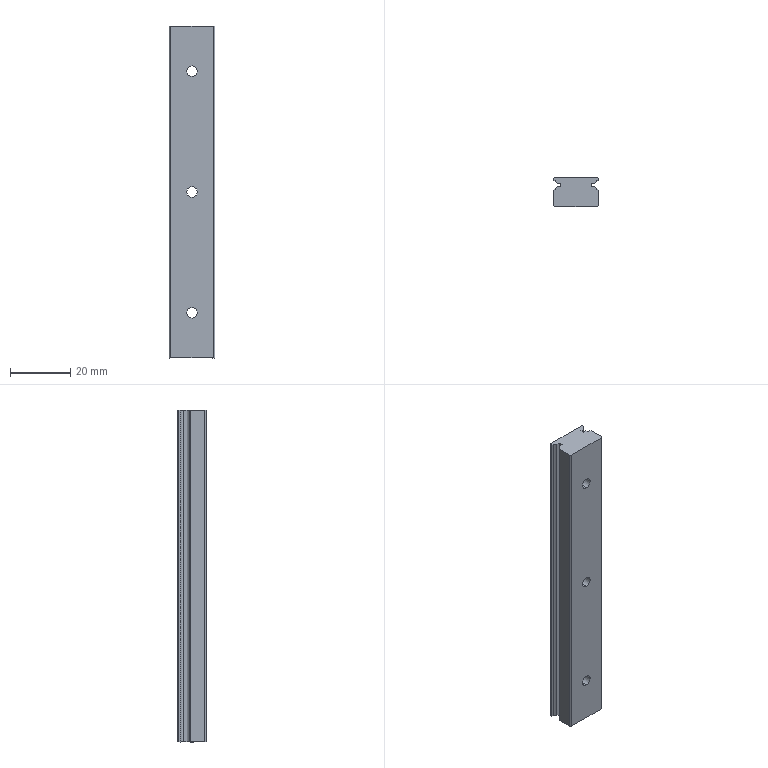Part | SolidWorks | features BaseBody 1 | 1 solid | 41 faces | box 15 x 9.5 x 110 mm | volume 14060 mm3 | plane 25 | cylinder 16 | commonest cylinder face diameters 3.5 x10 6 x6
STEP:
#1=CARTESIAN_POINT('',(0.,5.,-38.25));
#2=VERTEX_POINT('',#1);
#3=CARTESIAN_POINT('',(0.,5.,-41.75));
#4=VERTEX_POINT('',#3);
#5=CARTESIAN_POINT('',(0.,5.,-40.));
#6=DIRECTION('',(0.,-1.,0.));
#7=DIRECTION('',(0.,0.,-1.));
#8=AXIS2_PLACEMENT_3D('',#5,#6,#7);
#9=CIRCLE('',#8,1.75);
#10=EDGE_CURVE('',#2,#4,#9,.T.);
#11=ORIENTED_EDGE('',*,*,#10,.F.);
#12=CARTESIAN_POINT('',(0.,0.,-38.25));
#13=VERTEX_POINT('',#12);
#14=CARTESIAN_POINT('',(0.,2.5,-38.25));
#15=DIRECTION('',(0.,-1.,0.));
#16=VECTOR('',#15,1000.);
#17=LINE('',#14,#16);
#18=EDGE_CURVE('',#2,#13,#17,.T.);
#19=ORIENTED_EDGE('',*,*,#18,.T.);
#20=CARTESIAN_POINT('',(0.,0.,-41.75));
#21=VERTEX_POINT('',#20);
#22=CARTESIAN_POINT('',(0.,0.,-40.));
#23=DIRECTION('',(0.,1.,0.));
#24=DIRECTION('',(0.,0.,-1.));
#25=AXIS2_PLACEMENT_3D('',#22,#23,#24);
#26=CIRCLE('',#25,1.75);
#27=EDGE_CURVE('',#21,#13,#26,.T.);
#28=ORIENTED_EDGE('',*,*,#27,.F.);
#29=CARTESIAN_POINT('',(0.,2.5,-41.75));
#30=DIRECTION('',(0.,-1.,0.));
#31=VECTOR('',#30,1000.);
#32=LINE('',#29,#31);
#33=EDGE_CURVE('',#4,#21,#32,.T.);
#34=ORIENTED_EDGE('',*,*,#33,.F.);
#35=EDGE_LOOP('',(#11,#19,#28,#34));
#36=FACE_OUTER_BOUND('',#35,.T.);
#37=CARTESIAN_POINT('',(0.,2.5,-40.));
#38=DIRECTION('',(0.,-1.,0.));
#39=DIRECTION('',(0.,0.,-1.));
#40=AXIS2_PLACEMENT_3D('',#37,#38,#39);
#41=CYLINDRICAL_SURFACE('',#40,1.75);
#42=ADVANCED_FACE('',(#36),#41,.F.);
#43=CARTESIAN_POINT('',(0.,5.,41.75));
#44=VERTEX_POINT('',#43);
#45=CARTESIAN_POINT('',(0.,5.,38.25));
#46=VERTEX_POINT('',#45);
#47=CARTESIAN_POINT('',(0.,5.,40.));
#48=DIRECTION('',(0.,-1.,0.));
#49=DIRECTION('',(0.,0.,-1.));
#50=AXIS2_PLACEMENT_3D('',#47,#48,#49);
#51=CIRCLE('',#50,1.75);
#52=EDGE_CURVE('',#44,#46,#51,.T.);
#53=ORIENTED_EDGE('',*,*,#52,.F.);
#54=CARTESIAN_POINT('',(0.,0.,41.75));
#55=VERTEX_POINT('',#54);
#56=CARTESIAN_POINT('',(0.,2.5,41.75));
#57=DIRECTION('',(0.,-1.,0.));
#58=VECTOR('',#57,1000.);
#59=LINE('',#56,#58);
#60=EDGE_CURVE('',#44,#55,#59,.T.);
#61=ORIENTED_EDGE('',*,*,#60,.T.);
#62=CARTESIAN_POINT('',(0.,0.,38.25));
#63=VERTEX_POINT('',#62);
#64=CARTESIAN_POINT('',(0.,0.,40.));
#65=DIRECTION('',(0.,1.,0.));
#66=DIRECTION('',(0.,0.,-1.));
#67=AXIS2_PLACEMENT_3D('',#64,#65,#66);
#68=CIRCLE('',#67,1.75);
#69=EDGE_CURVE('',#63,#55,#68,.T.);
#70=ORIENTED_EDGE('',*,*,#69,.F.);
#71=CARTESIAN_POINT('',(0.,2.5,38.25));
#72=DIRECTION('',(0.,-1.,0.));
#73=VECTOR('',#72,1000.);
#74=LINE('',#71,#73);
#75=EDGE_CURVE('',#46,#63,#74,.T.);
#76=ORIENTED_EDGE('',*,*,#75,.F.);
#77=EDGE_LOOP('',(#53,#61,#70,#76));
#78=FACE_OUTER_BOUND('',#77,.T.);
#79=CARTESIAN_POINT('',(0.,2.5,40.));
#80=DIRECTION('',(0.,-1.,0.));
#81=DIRECTION('',(0.,0.,-1.));
#82=AXIS2_PLACEMENT_3D('',#79,#80,#81);
#83=CYLINDRICAL_SURFACE('',#82,1.75);
#84=ADVANCED_FACE('',(#78),#83,.F.);
#85=CARTESIAN_POINT('',(0.,5.,1.75));
#86=VERTEX_POINT('',#85);
#87=CARTESIAN_POINT('',(0.,5.,-1.75));
#88=VERTEX_POINT('',#87);
#89=CARTESIAN_POINT('',(0.,5.,0.));
#90=DIRECTION('',(0.,-1.,0.));
#91=DIRECTION('',(0.,0.,-1.));
#92=AXIS2_PLACEMENT_3D('',#89,#90,#91);
#93=CIRCLE('',#92,1.75);
#94=EDGE_CURVE('',#86,#88,#93,.T.);
#95=ORIENTED_EDGE('',*,*,#94,.F.);
#96=CARTESIAN_POINT('',(0.,0.,1.75));
#97=VERTEX_POINT('',#96);
#98=CARTESIAN_POINT('',(0.,2.5,1.75));
#99=DIRECTION('',(0.,-1.,0.));
#100=VECTOR('',#99,1000.);
#101=LINE('',#98,#100);
#102=EDGE_CURVE('',#86,#97,#101,.T.);
#103=ORIENTED_EDGE('',*,*,#102,.T.);
#104=CARTESIAN_POINT('',(0.,0.,-1.75));
#105=VERTEX_POINT('',#104);
#106=CARTESIAN_POINT('',(0.,0.,0.));
#107=DIRECTION('',(0.,1.,0.));
#108=DIRECTION('',(0.,0.,-1.));
#109=AXIS2_PLACEMENT_3D('',#106,#107,#108);
#110=CIRCLE('',#109,1.75);
#111=EDGE_CURVE('',#105,#97,#110,.T.);
#112=ORIENTED_EDGE('',*,*,#111,.F.);
#113=CARTESIAN_POINT('',(0.,2.5,-1.75));
#114=DIRECTION('',(0.,-1.,0.));
#115=VECTOR('',#114,1000.);
#116=LINE('',#113,#115);
#117=EDGE_CURVE('',#88,#105,#116,.T.);
#118=ORIENTED_EDGE('',*,*,#117,.F.);
#119=EDGE_LOOP('',(#95,#103,#112,#118));
#120=FACE_OUTER_BOUND('',#119,.T.);
#121=CARTESIAN_POINT('',(0.,2.5,0.));
#122=DIRECTION('',(0.,-1.,0.));
#123=DIRECTION('',(0.,0.,-1.));
#124=AXIS2_PLACEMENT_3D('',#121,#122,#123);
#125=CYLINDRICAL_SURFACE('',#124,1.75);
#126=ADVANCED_FACE('',(#120),#125,.F.);
#127=CARTESIAN_POINT('',(0.,9.5,-37.));
#128=VERTEX_POINT('',#127);
#129=CARTESIAN_POINT('',(0.,9.5,-43.));
#130=VERTEX_POINT('',#129);
#131=CARTESIAN_POINT('',(0.,9.5,-40.));
#132=DIRECTION('',(0.,-1.,0.));
#133=DIRECTION('',(0.,0.,-1.));
#134=AXIS2_PLACEMENT_3D('',#131,#132,#133);
#135=CIRCLE('',#134,3.);
#136=EDGE_CURVE('',#128,#130,#135,.T.);
#137=ORIENTED_EDGE('',*,*,#136,.F.);
#138=CARTESIAN_POINT('',(0.,5.,-37.));
#139=VERTEX_POINT('',#138);
#140=CARTESIAN_POINT('',(0.,7.25,-37.));
#141=DIRECTION('',(0.,-1.,0.));
#142=VECTOR('',#141,1000.);
#143=LINE('',#140,#142);
#144=EDGE_CURVE('',#128,#139,#143,.T.);
#145=ORIENTED_EDGE('',*,*,#144,.T.);
#146=CARTESIAN_POINT('',(0.,5.,-43.));
#147=VERTEX_POINT('',#146);
#148=CARTESIAN_POINT('',(0.,5.,-40.));
#149=DIRECTION('',(0.,-1.,0.));
#150=DIRECTION('',(0.,0.,-1.));
#151=AXIS2_PLACEMENT_3D('',#148,#149,#150);
#152=CIRCLE('',#151,3.);
#153=EDGE_CURVE('',#139,#147,#152,.T.);
#154=ORIENTED_EDGE('',*,*,#153,.T.);
#155=CARTESIAN_POINT('',(0.,7.25,-43.));
#156=DIRECTION('',(0.,-1.,0.));
#157=VECTOR('',#156,1000.);
#158=LINE('',#155,#157);
#159=EDGE_CURVE('',#130,#147,#158,.T.);
#160=ORIENTED_EDGE('',*,*,#159,.F.);
#161=EDGE_LOOP('',(#137,#145,#154,#160));
#162=FACE_OUTER_BOUND('',#161,.T.);
#163=CARTESIAN_POINT('',(0.,7.25,-40.));
#164=DIRECTION('',(0.,-1.,0.));
#165=DIRECTION('',(0.,0.,-1.));
#166=AXIS2_PLACEMENT_3D('',#163,#164,#165);
#167=CYLINDRICAL_SURFACE('',#166,3.);
#168=ADVANCED_FACE('',(#162),#167,.F.);
#169=CARTESIAN_POINT('',(0.,9.5,43.));
#170=VERTEX_POINT('',#169);
#171=CARTESIAN_POINT('',(0.,9.5,37.));
#172=VERTEX_POINT('',#171);
#173=CARTESIAN_POINT('',(0.,9.5,40.));
#174=DIRECTION('',(0.,-1.,0.));
#175=DIRECTION('',(0.,0.,-1.));
#176=AXIS2_PLACEMENT_3D('',#173,#174,#175);
#177=CIRCLE('',#176,3.);
#178=EDGE_CURVE('',#170,#172,#177,.T.);
#179=ORIENTED_EDGE('',*,*,#178,.F.);
#180=CARTESIAN_POINT('',(0.,5.,43.));
#181=VERTEX_POINT('',#180);
#182=CARTESIAN_POINT('',(0.,7.25,43.));
#183=DIRECTION('',(0.,-1.,0.));
#184=VECTOR('',#183,1000.);
#185=LINE('',#182,#184);
#186=EDGE_CURVE('',#170,#181,#185,.T.);
#187=ORIENTED_EDGE('',*,*,#186,.T.);
#188=CARTESIAN_POINT('',(0.,5.,37.));
#189=VERTEX_POINT('',#188);
#190=CARTESIAN_POINT('',(0.,5.,40.));
#191=DIRECTION('',(0.,-1.,0.));
#192=DIRECTION('',(0.,0.,-1.));
#193=AXIS2_PLACEMENT_3D('',#190,#191,#192);
#194=CIRCLE('',#193,3.);
#195=EDGE_CURVE('',#181,#189,#194,.T.);
#196=ORIENTED_EDGE('',*,*,#195,.T.);
#197=CARTESIAN_POINT('',(0.,7.25,37.));
#198=DIRECTION('',(0.,-1.,0.));
#199=VECTOR('',#198,1000.);
#200=LINE('',#197,#199);
#201=EDGE_CURVE('',#172,#189,#200,.T.);
#202=ORIENTED_EDGE('',*,*,#201,.F.);
#203=EDGE_LOOP('',(#179,#187,#196,#202));
#204=FACE_OUTER_BOUND('',#203,.T.);
#205=CARTESIAN_POINT('',(0.,7.25,40.));
#206=DIRECTION('',(0.,-1.,0.));
#207=DIRECTION('',(0.,0.,-1.));
#208=AXIS2_PLACEMENT_3D('',#205,#206,#207);
#209=CYLINDRICAL_SURFACE('',#208,3.);
#210=ADVANCED_FACE('',(#204),#209,.F.);
#211=CARTESIAN_POINT('',(0.,9.5,3.));
#212=VERTEX_POINT('',#211);
#213=CARTESIAN_POINT('',(0.,9.5,-3.));
#214=VERTEX_POINT('',#213);
#215=CARTESIAN_POINT('',(0.,9.5,0.));
#216=DIRECTION('',(0.,-1.,0.));
#217=DIRECTION('',(0.,0.,-1.));
#218=AXIS2_PLACEMENT_3D('',#215,#216,#217);
#219=CIRCLE('',#218,3.);
#220=EDGE_CURVE('',#212,#214,#219,.T.);
#221=ORIENTED_EDGE('',*,*,#220,.F.);
#222=CARTESIAN_POINT('',(0.,5.,3.));
#223=VERTEX_POINT('',#222);
#224=CARTESIAN_POINT('',(0.,7.25,3.));
#225=DIRECTION('',(0.,-1.,0.));
#226=VECTOR('',#225,1000.);
#227=LINE('',#224,#226);
#228=EDGE_CURVE('',#212,#223,#227,.T.);
#229=ORIENTED_EDGE('',*,*,#228,.T.);
#230=CARTESIAN_POINT('',(0.,5.,-3.));
#231=VERTEX_POINT('',#230);
#232=CARTESIAN_POINT('',(0.,5.,0.));
#233=DIRECTION('',(0.,-1.,0.));
#234=DIRECTION('',(0.,0.,-1.));
#235=AXIS2_PLACEMENT_3D('',#232,#233,#234);
#236=CIRCLE('',#235,3.);
#237=EDGE_CURVE('',#223,#231,#236,.T.);
#238=ORIENTED_EDGE('',*,*,#237,.T.);
#239=CARTESIAN_POINT('',(0.,7.25,-3.));
#240=DIRECTION('',(0.,-1.,0.));
#241=VECTOR('',#240,1000.);
#242=LINE('',#239,#241);
#243=EDGE_CURVE('',#214,#231,#242,.T.);
#244=ORIENTED_EDGE('',*,*,#243,.F.);
#245=EDGE_LOOP('',(#221,#229,#238,#244));
#246=FACE_OUTER_BOUND('',#245,.T.);
#247=CARTESIAN_POINT('',(0.,7.25,0.));
#248=DIRECTION('',(0.,-1.,0.));
#249=DIRECTION('',(0.,0.,-1.));
#250=AXIS2_PLACEMENT_3D('',#247,#248,#249);
#251=CYLINDRICAL_SURFACE('',#250,3.);
#252=ADVANCED_FACE('',(#246),#251,.F.);
#253=CARTESIAN_POINT('',(7.,0.,55.));
#254=VERTEX_POINT('',#253);
#255=CARTESIAN_POINT('',(-7.,0.,55.));
#256=VERTEX_POINT('',#255);
#257=CARTESIAN_POINT('',(-7.,0.,55.));
#258=DIRECTION('',(-1.,0.,0.));
#259=VECTOR('',#258,1000.);
#260=LINE('',#257,#259);
#261=EDGE_CURVE('',#254,#256,#260,.T.);
#262=ORIENTED_EDGE('',*,*,#261,.T.);
#263=CARTESIAN_POINT('',(-7.,0.,-55.));
#264=VERTEX_POINT('',#263);
#265=CARTESIAN_POINT('',(-7.,0.,55.));
#266=DIRECTION('',(0.,0.,-1.));
#267=VECTOR('',#266,1000.);
#268=LINE('',#265,#267);
#269=EDGE_CURVE('',#256,#264,#268,.T.);
#270=ORIENTED_EDGE('',*,*,#269,.T.);
#271=CARTESIAN_POINT('',(7.,0.,-55.));
#272=VERTEX_POINT('',#271);
#273=CARTESIAN_POINT('',(-7.,0.,-55.));
#274=DIRECTION('',(1.,0.,0.));
#275=VECTOR('',#274,1000.);
#276=LINE('',#273,#275);
#277=EDGE_CURVE('',#264,#272,#276,.T.);
#278=ORIENTED_EDGE('',*,*,#277,.T.);
#279=CARTESIAN_POINT('',(7.,0.,55.));
#280=DIRECTION('',(0.,0.,1.));
#281=VECTOR('',#280,1000.);
#282=LINE('',#279,#281);
#283=EDGE_CURVE('',#272,#254,#282,.T.);
#284=ORIENTED_EDGE('',*,*,#283,.T.);
#285=EDGE_LOOP('',(#262,#270,#278,#284));
#286=FACE_OUTER_BOUND('',#285,.T.);
#287=ORIENTED_EDGE('',*,*,#27,.T.);
#288=CARTESIAN_POINT('',(0.,0.,-40.));
#289=DIRECTION('',(0.,1.,0.));
#290=DIRECTION('',(0.,0.,-1.));
#291=AXIS2_PLACEMENT_3D('',#288,#289,#290);
#292=CIRCLE('',#291,1.75);
#293=EDGE_CURVE('',#13,#21,#292,.T.);
#294=ORIENTED_EDGE('',*,*,#293,.T.);
#295=EDGE_LOOP('',(#287,#294));
#296=FACE_BOUND('',#295,.T.);
#297=ORIENTED_EDGE('',*,*,#69,.T.);
#298=CARTESIAN_POINT('',(0.,0.,40.));
#299=DIRECTION('',(0.,1.,0.));
#300=DIRECTION('',(0.,0.,-1.));
#301=AXIS2_PLACEMENT_3D('',#298,#299,#300);
#302=CIRCLE('',#301,1.75);
#303=EDGE_CURVE('',#55,#63,#302,.T.);
#304=ORIENTED_EDGE('',*,*,#303,.T.);
#305=EDGE_LOOP('',(#297,#304));
#306=FACE_BOUND('',#305,.T.);
#307=ORIENTED_EDGE('',*,*,#111,.T.);
#308=CARTESIAN_POINT('',(0.,0.,0.));
#309=DIRECTION('',(0.,1.,0.));
#310=DIRECTION('',(0.,0.,-1.));
#311=AXIS2_PLACEMENT_3D('',#308,#309,#310);
#312=CIRCLE('',#311,1.75);
#313=EDGE_CURVE('',#97,#105,#312,.T.);
#314=ORIENTED_EDGE('',*,*,#313,.T.);
#315=EDGE_LOOP('',(#307,#314));
#316=FACE_BOUND('',#315,.T.);
#317=CARTESIAN_POINT('',(-7.,0.,55.));
#318=DIRECTION('',(0.,-1.,0.));
#319=DIRECTION('',(0.,0.,-1.));
#320=AXIS2_PLACEMENT_3D('',#317,#318,#319);
#321=PLANE('',#320);
#322=ADVANCED_FACE('',(#286,#296,#306,#316),#321,.T.);
#323=CARTESIAN_POINT('',(-7.5,0.5,55.));
#324=VERTEX_POINT('',#323);
#325=CARTESIAN_POINT('',(-7.5,0.5,55.));
#326=DIRECTION('',(-0.7071,0.7071,0.));
#327=VECTOR('',#326,1000.);
#328=LINE('',#325,#327);
#329=EDGE_CURVE('',#256,#324,#328,.T.);
#330=ORIENTED_EDGE('',*,*,#329,.T.);
#331=CARTESIAN_POINT('',(-7.5,0.5,-55.));
#332=VERTEX_POINT('',#331);
#333=CARTESIAN_POINT('',(-7.5,0.5,55.));
#334=DIRECTION('',(0.,0.,-1.));
#335=VECTOR('',#334,1000.);
#336=LINE('',#333,#335);
#337=EDGE_CURVE('',#324,#332,#336,.T.);
#338=ORIENTED_EDGE('',*,*,#337,.T.);
#339=CARTESIAN_POINT('',(-7.5,0.5,-55.));
#340=DIRECTION('',(0.7071,-0.7071,0.));
#341=VECTOR('',#340,1000.);
#342=LINE('',#339,#341);
#343=EDGE_CURVE('',#332,#264,#342,.T.);
#344=ORIENTED_EDGE('',*,*,#343,.T.);
#345=ORIENTED_EDGE('',*,*,#269,.F.);
#346=EDGE_LOOP('',(#330,#338,#344,#345));
#347=FACE_OUTER_BOUND('',#346,.T.);
#348=CARTESIAN_POINT('',(-7.5,0.5,55.));
#349=DIRECTION('',(-0.7071,-0.7071,0.));
#350=DIRECTION('',(0.7071,-0.7071,0.));
#351=AXIS2_PLACEMENT_3D('',#348,#349,#350);
#352=PLANE('',#351);
#353=ADVANCED_FACE('',(#347),#352,.T.);
#354=CARTESIAN_POINT('',(-6.218,6.4,55.));
#355=VERTEX_POINT('',#354);
#356=CARTESIAN_POINT('',(-6.94,5.599,55.));
#357=VERTEX_POINT('',#356);
#358=CARTESIAN_POINT('',(-7.815,7.115,55.));
#359=DIRECTION('',(0.,0.,-1.));
#360=DIRECTION('',(1.,0.,0.));
#361=AXIS2_PLACEMENT_3D('',#358,#359,#360);
#362=CIRCLE('',#361,1.75);
#363=EDGE_CURVE('',#355,#357,#362,.T.);
#364=ORIENTED_EDGE('',*,*,#363,.T.);
#365=CARTESIAN_POINT('',(-7.5,5.276,55.));
#366=VERTEX_POINT('',#365);
#367=CARTESIAN_POINT('',(-6.94,5.599,55.));
#368=DIRECTION('',(0.866,0.5,0.));
#369=VECTOR('',#368,1000.);
#370=LINE('',#367,#369);
#371=EDGE_CURVE('',#366,#357,#370,.T.);
#372=ORIENTED_EDGE('',*,*,#371,.F.);
#373=CARTESIAN_POINT('',(-7.5,0.,55.));
#374=DIRECTION('',(0.,-1.,0.));
#375=VECTOR('',#374,1000.);
#376=LINE('',#373,#375);
#377=EDGE_CURVE('',#366,#324,#376,.T.);
#378=ORIENTED_EDGE('',*,*,#377,.T.);
#379=ORIENTED_EDGE('',*,*,#329,.F.);
#380=ORIENTED_EDGE('',*,*,#261,.F.);
#381=CARTESIAN_POINT('',(7.5,0.5,55.));
#382=VERTEX_POINT('',#381);
#383=CARTESIAN_POINT('',(7.,0.,55.));
#384=DIRECTION('',(0.7071,0.7071,0.));
#385=VECTOR('',#384,1000.);
#386=LINE('',#383,#385);
#387=EDGE_CURVE('',#254,#382,#386,.T.);
#388=ORIENTED_EDGE('',*,*,#387,.T.);
#389=CARTESIAN_POINT('',(7.5,5.276,55.));
#390=VERTEX_POINT('',#389);
#391=CARTESIAN_POINT('',(7.5,0.,55.));
#392=DIRECTION('',(0.,1.,0.));
#393=VECTOR('',#392,1000.);
#394=LINE('',#391,#393);
#395=EDGE_CURVE('',#382,#390,#394,.T.);
#396=ORIENTED_EDGE('',*,*,#395,.T.);
#397=CARTESIAN_POINT('',(6.94,5.599,55.));
#398=VERTEX_POINT('',#397);
#399=CARTESIAN_POINT('',(7.5,5.276,55.));
#400=DIRECTION('',(0.866,-0.5,0.));
#401=VECTOR('',#400,1000.);
#402=LINE('',#399,#401);
#403=EDGE_CURVE('',#398,#390,#402,.T.);
#404=ORIENTED_EDGE('',*,*,#403,.F.);
#405=CARTESIAN_POINT('',(6.218,6.4,55.));
#406=VERTEX_POINT('',#405);
#407=CARTESIAN_POINT('',(7.815,7.115,55.));
#408=DIRECTION('',(0.,0.,-1.));
#409=DIRECTION('',(1.,0.,0.));
#410=AXIS2_PLACEMENT_3D('',#407,#408,#409);
#411=CIRCLE('',#410,1.75);
#412=EDGE_CURVE('',#398,#406,#411,.T.);
#413=ORIENTED_EDGE('',*,*,#412,.T.);
#414=CARTESIAN_POINT('',(5.,6.4,55.));
#415=VERTEX_POINT('',#414);
#416=CARTESIAN_POINT('',(6.218,6.4,55.));
#417=DIRECTION('',(1.,0.,0.));
#418=VECTOR('',#417,1000.);
#419=LINE('',#416,#418);
#420=EDGE_CURVE('',#415,#406,#419,.T.);
#421=ORIENTED_EDGE('',*,*,#420,.F.);
#422=CARTESIAN_POINT('',(5.,7.6,55.));
#423=VERTEX_POINT('',#422);
#424=CARTESIAN_POINT('',(5.,6.4,55.));
#425=DIRECTION('',(0.,-1.,0.));
#426=VECTOR('',#425,1000.);
#427=LINE('',#424,#426);
#428=EDGE_CURVE('',#423,#415,#427,.T.);
#429=ORIENTED_EDGE('',*,*,#428,.F.);
#430=CARTESIAN_POINT('',(6.218,7.6,55.));
#431=VERTEX_POINT('',#430);
#432=CARTESIAN_POINT('',(5.,7.6,55.));
#433=DIRECTION('',(-1.,0.,0.));
#434=VECTOR('',#433,1000.);
#435=LINE('',#432,#434);
#436=EDGE_CURVE('',#431,#423,#435,.T.);
#437=ORIENTED_EDGE('',*,*,#436,.F.);
#438=CARTESIAN_POINT('',(6.94,8.401,55.));
#439=VERTEX_POINT('',#438);
#440=CARTESIAN_POINT('',(7.815,6.885,55.));
#441=DIRECTION('',(0.,0.,-1.));
#442=DIRECTION('',(1.,0.,0.));
#443=AXIS2_PLACEMENT_3D('',#440,#441,#442);
#444=CIRCLE('',#443,1.75);
#445=EDGE_CURVE('',#431,#439,#444,.T.);
#446=ORIENTED_EDGE('',*,*,#445,.T.);
#447=CARTESIAN_POINT('',(7.5,8.724,55.));
#448=VERTEX_POINT('',#447);
#449=CARTESIAN_POINT('',(6.94,8.401,55.));
#450=DIRECTION('',(-0.866,-0.5,0.));
#451=VECTOR('',#450,1000.);
#452=LINE('',#449,#451);
#453=EDGE_CURVE('',#448,#439,#452,.T.);
#454=ORIENTED_EDGE('',*,*,#453,.F.);
#455=CARTESIAN_POINT('',(7.5,9.2,55.));
#456=VERTEX_POINT('',#455);
#457=CARTESIAN_POINT('',(7.5,8.724,55.));
#458=DIRECTION('',(0.,-1.,0.));
#459=VECTOR('',#458,1000.);
#460=LINE('',#457,#459);
#461=EDGE_CURVE('',#456,#448,#460,.T.);
#462=ORIENTED_EDGE('',*,*,#461,.F.);
#463=CARTESIAN_POINT('',(7.2,9.5,55.));
#464=VERTEX_POINT('',#463);
#465=CARTESIAN_POINT('',(7.5,9.2,55.));
#466=DIRECTION('',(0.7071,-0.7071,0.));
#467=VECTOR('',#466,1000.);
#468=LINE('',#465,#467);
#469=EDGE_CURVE('',#464,#456,#468,.T.);
#470=ORIENTED_EDGE('',*,*,#469,.F.);
#471=CARTESIAN_POINT('',(-7.2,9.5,55.));
#472=VERTEX_POINT('',#471);
#473=CARTESIAN_POINT('',(0.,9.5,55.));
#474=DIRECTION('',(-1.,0.,0.));
#475=VECTOR('',#474,1000.);
#476=LINE('',#473,#475);
#477=EDGE_CURVE('',#464,#472,#476,.T.);
#478=ORIENTED_EDGE('',*,*,#477,.T.);
#479=CARTESIAN_POINT('',(-7.5,9.2,55.));
#480=VERTEX_POINT('',#479);
#481=CARTESIAN_POINT('',(-7.2,9.5,55.));
#482=DIRECTION('',(0.7071,0.7071,0.));
#483=VECTOR('',#482,1000.);
#484=LINE('',#481,#483);
#485=EDGE_CURVE('',#480,#472,#484,.T.);
#486=ORIENTED_EDGE('',*,*,#485,.F.);
#487=CARTESIAN_POINT('',(-7.5,8.724,55.));
#488=VERTEX_POINT('',#487);
#489=CARTESIAN_POINT('',(-7.5,9.2,55.));
#490=DIRECTION('',(0.,1.,0.));
#491=VECTOR('',#490,1000.);
#492=LINE('',#489,#491);
#493=EDGE_CURVE('',#488,#480,#492,.T.);
#494=ORIENTED_EDGE('',*,*,#493,.F.);
#495=CARTESIAN_POINT('',(-6.94,8.401,55.));
#496=VERTEX_POINT('',#495);
#497=CARTESIAN_POINT('',(-7.5,8.724,55.));
#498=DIRECTION('',(-0.866,0.5,0.));
#499=VECTOR('',#498,1000.);
#500=LINE('',#497,#499);
#501=EDGE_CURVE('',#496,#488,#500,.T.);
#502=ORIENTED_EDGE('',*,*,#501,.F.);
#503=CARTESIAN_POINT('',(-6.218,7.6,55.));
#504=VERTEX_POINT('',#503);
#505=CARTESIAN_POINT('',(-7.815,6.885,55.));
#506=DIRECTION('',(0.,0.,-1.));
#507=DIRECTION('',(1.,0.,0.));
#508=AXIS2_PLACEMENT_3D('',#505,#506,#507);
#509=CIRCLE('',#508,1.75);
#510=EDGE_CURVE('',#496,#504,#509,.T.);
#511=ORIENTED_EDGE('',*,*,#510,.T.);
#512=CARTESIAN_POINT('',(-5.,7.6,55.));
#513=VERTEX_POINT('',#512);
#514=CARTESIAN_POINT('',(-6.218,7.6,55.));
#515=DIRECTION('',(-1.,0.,0.));
#516=VECTOR('',#515,1000.);
#517=LINE('',#514,#516);
#518=EDGE_CURVE('',#513,#504,#517,.T.);
#519=ORIENTED_EDGE('',*,*,#518,.F.);
#520=CARTESIAN_POINT('',(-5.,6.4,55.));
#521=VERTEX_POINT('',#520);
#522=CARTESIAN_POINT('',(-5.,7.6,55.));
#523=DIRECTION('',(0.,1.,0.));
#524=VECTOR('',#523,1000.);
#525=LINE('',#522,#524);
#526=EDGE_CURVE('',#521,#513,#525,.T.);
#527=ORIENTED_EDGE('',*,*,#526,.F.);
#528=CARTESIAN_POINT('',(-5.,6.4,55.));
#529=DIRECTION('',(1.,0.,0.));
#530=VECTOR('',#529,1000.);
#531=LINE('',#528,#530);
#532=EDGE_CURVE('',#355,#521,#531,.T.);
#533=ORIENTED_EDGE('',*,*,#532,.F.);
#534=EDGE_LOOP('',(#364,#372,#378,#379,#380,#388,#396,#404,#413,#421,#429,#437,#446,#454,#462,#470,#478,#486,#494,#502,#511,#519,#527,#533));
#535=FACE_OUTER_BOUND('',#534,.T.);
#536=CARTESIAN_POINT('',(0.,0.,55.));
#537=DIRECTION('',(0.,0.,1.));
#538=DIRECTION('',(1.,0.,0.));
#539=AXIS2_PLACEMENT_3D('',#536,#537,#538);
#540=PLANE('',#539);
#541=ADVANCED_FACE('',(#535),#540,.T.);
#542=ORIENTED_EDGE('',*,*,#387,.F.);
#543=ORIENTED_EDGE('',*,*,#283,.F.);
#544=CARTESIAN_POINT('',(7.5,0.5,-55.));
#545=VERTEX_POINT('',#544);
#546=CARTESIAN_POINT('',(7.,0.,-55.));
#547=DIRECTION('',(0.7071,0.7071,0.));
#548=VECTOR('',#547,1000.);
#549=LINE('',#546,#548);
#550=EDGE_CURVE('',#272,#545,#549,.T.);
#551=ORIENTED_EDGE('',*,*,#550,.T.);
#552=CARTESIAN_POINT('',(7.5,0.5,55.));
#553=DIRECTION('',(0.,0.,1.));
#554=VECTOR('',#553,1000.);
#555=LINE('',#552,#554);
#556=EDGE_CURVE('',#545,#382,#555,.T.);
#557=ORIENTED_EDGE('',*,*,#556,.T.);
#558=EDGE_LOOP('',(#542,#543,#551,#557));
#559=FACE_OUTER_BOUND('',#558,.T.);
#560=CARTESIAN_POINT('',(7.,0.,55.));
#561=DIRECTION('',(0.7071,-0.7071,0.));
#562=DIRECTION('',(0.7071,0.7071,0.));
#563=AXIS2_PLACEMENT_3D('',#560,#561,#562);
#564=PLANE('',#563);
#565=ADVANCED_FACE('',(#559),#564,.T.);
#566=CARTESIAN_POINT('',(-7.5,5.276,-55.));
#567=VERTEX_POINT('',#566);
#568=CARTESIAN_POINT('',(-7.5,0.,-55.));
#569=DIRECTION('',(0.,-1.,0.));
#570=VECTOR('',#569,1000.);
#571=LINE('',#568,#570);
#572=EDGE_CURVE('',#567,#332,#571,.T.);
#573=ORIENTED_EDGE('',*,*,#572,.F.);
#574=CARTESIAN_POINT('',(-6.94,5.599,-55.));
#575=VERTEX_POINT('',#574);
#576=CARTESIAN_POINT('',(-6.94,5.599,-55.));
#577=DIRECTION('',(-0.866,-0.5,0.));
#578=VECTOR('',#577,1000.);
#579=LINE('',#576,#578);
#580=EDGE_CURVE('',#575,#567,#579,.T.);
#581=ORIENTED_EDGE('',*,*,#580,.F.);
#582=CARTESIAN_POINT('',(-6.218,6.4,-55.));
#583=VERTEX_POINT('',#582);
#584=CARTESIAN_POINT('',(-7.815,7.115,-55.));
#585=DIRECTION('',(0.,0.,1.));
#586=DIRECTION('',(1.,0.,0.));
#587=AXIS2_PLACEMENT_3D('',#584,#585,#586);
#588=CIRCLE('',#587,1.75);
#589=EDGE_CURVE('',#575,#583,#588,.T.);
#590=ORIENTED_EDGE('',*,*,#589,.T.);
#591=CARTESIAN_POINT('',(-5.,6.4,-55.));
#592=VERTEX_POINT('',#591);
#593=CARTESIAN_POINT('',(-5.,6.4,-55.));
#594=DIRECTION('',(-1.,0.,0.));
#595=VECTOR('',#594,1000.);
#596=LINE('',#593,#595);
#597=EDGE_CURVE('',#592,#583,#596,.T.);
#598=ORIENTED_EDGE('',*,*,#597,.F.);
#599=CARTESIAN_POINT('',(-5.,7.6,-55.));
#600=VERTEX_POINT('',#599);
#601=CARTESIAN_POINT('',(-5.,7.6,-55.));
#602=DIRECTION('',(0.,-1.,0.));
#603=VECTOR('',#602,1000.);
#604=LINE('',#601,#603);
#605=EDGE_CURVE('',#600,#592,#604,.T.);
#606=ORIENTED_EDGE('',*,*,#605,.F.);
#607=CARTESIAN_POINT('',(-6.218,7.6,-55.));
#608=VERTEX_POINT('',#607);
#609=CARTESIAN_POINT('',(-6.218,7.6,-55.));
#610=DIRECTION('',(1.,0.,0.));
#611=VECTOR('',#610,1000.);
#612=LINE('',#609,#611);
#613=EDGE_CURVE('',#608,#600,#612,.T.);
#614=ORIENTED_EDGE('',*,*,#613,.F.);
#615=CARTESIAN_POINT('',(-6.94,8.401,-55.));
#616=VERTEX_POINT('',#615);
#617=CARTESIAN_POINT('',(-7.815,6.885,-55.));
#618=DIRECTION('',(0.,0.,1.));
#619=DIRECTION('',(1.,0.,0.));
#620=AXIS2_PLACEMENT_3D('',#617,#618,#619);
#621=CIRCLE('',#620,1.75);
#622=EDGE_CURVE('',#608,#616,#621,.T.);
#623=ORIENTED_EDGE('',*,*,#622,.T.);
#624=CARTESIAN_POINT('',(-7.5,8.724,-55.));
#625=VERTEX_POINT('',#624);
#626=CARTESIAN_POINT('',(-7.5,8.724,-55.));
#627=DIRECTION('',(0.866,-0.5,0.));
#628=VECTOR('',#627,1000.);
#629=LINE('',#626,#628);
#630=EDGE_CURVE('',#625,#616,#629,.T.);
#631=ORIENTED_EDGE('',*,*,#630,.F.);
#632=CARTESIAN_POINT('',(-7.5,9.2,-55.));
#633=VERTEX_POINT('',#632);
#634=CARTESIAN_POINT('',(-7.5,9.2,-55.));
#635=DIRECTION('',(0.,-1.,0.));
#636=VECTOR('',#635,1000.);
#637=LINE('',#634,#636);
#638=EDGE_CURVE('',#633,#625,#637,.T.);
#639=ORIENTED_EDGE('',*,*,#638,.F.);
#640=CARTESIAN_POINT('',(-7.2,9.5,-55.));
#641=VERTEX_POINT('',#640);
#642=CARTESIAN_POINT('',(-7.2,9.5,-55.));
#643=DIRECTION('',(-0.7071,-0.7071,0.));
#644=VECTOR('',#643,1000.);
#645=LINE('',#642,#644);
#646=EDGE_CURVE('',#641,#633,#645,.T.);
#647=ORIENTED_EDGE('',*,*,#646,.F.);
#648=CARTESIAN_POINT('',(7.2,9.5,-55.));
#649=VERTEX_POINT('',#648);
#650=CARTESIAN_POINT('',(0.,9.5,-55.));
#651=DIRECTION('',(-1.,0.,0.));
#652=VECTOR('',#651,1000.);
#653=LINE('',#650,#652);
#654=EDGE_CURVE('',#649,#641,#653,.T.);
#655=ORIENTED_EDGE('',*,*,#654,.F.);
#656=CARTESIAN_POINT('',(7.5,9.2,-55.));
#657=VERTEX_POINT('',#656);
#658=CARTESIAN_POINT('',(7.5,9.2,-55.));
#659=DIRECTION('',(-0.7071,0.7071,0.));
#660=VECTOR('',#659,1000.);
#661=LINE('',#658,#660);
#662=EDGE_CURVE('',#657,#649,#661,.T.);
#663=ORIENTED_EDGE('',*,*,#662,.F.);
#664=CARTESIAN_POINT('',(7.5,8.724,-55.));
#665=VERTEX_POINT('',#664);
#666=CARTESIAN_POINT('',(7.5,8.724,-55.));
#667=DIRECTION('',(0.,1.,0.));
#668=VECTOR('',#667,1000.);
#669=LINE('',#666,#668);
#670=EDGE_CURVE('',#665,#657,#669,.T.);
#671=ORIENTED_EDGE('',*,*,#670,.F.);
#672=CARTESIAN_POINT('',(6.94,8.401,-55.));
#673=VERTEX_POINT('',#672);
#674=CARTESIAN_POINT('',(6.94,8.401,-55.));
#675=DIRECTION('',(0.866,0.5,0.));
#676=VECTOR('',#675,1000.);
#677=LINE('',#674,#676);
#678=EDGE_CURVE('',#673,#665,#677,.T.);
#679=ORIENTED_EDGE('',*,*,#678,.F.);
#680=CARTESIAN_POINT('',(6.218,7.6,-55.));
#681=VERTEX_POINT('',#680);
#682=CARTESIAN_POINT('',(7.815,6.885,-55.));
#683=DIRECTION('',(0.,0.,1.));
#684=DIRECTION('',(1.,0.,0.));
#685=AXIS2_PLACEMENT_3D('',#682,#683,#684);
#686=CIRCLE('',#685,1.75);
#687=EDGE_CURVE('',#673,#681,#686,.T.);
#688=ORIENTED_EDGE('',*,*,#687,.T.);
#689=CARTESIAN_POINT('',(5.,7.6,-55.));
#690=VERTEX_POINT('',#689);
#691=CARTESIAN_POINT('',(5.,7.6,-55.));
#692=DIRECTION('',(1.,0.,0.));
#693=VECTOR('',#692,1000.);
#694=LINE('',#691,#693);
#695=EDGE_CURVE('',#690,#681,#694,.T.);
#696=ORIENTED_EDGE('',*,*,#695,.F.);
#697=CARTESIAN_POINT('',(5.,6.4,-55.));
#698=VERTEX_POINT('',#697);
#699=CARTESIAN_POINT('',(5.,6.4,-55.));
#700=DIRECTION('',(0.,1.,0.));
#701=VECTOR('',#700,1000.);
#702=LINE('',#699,#701);
#703=EDGE_CURVE('',#698,#690,#702,.T.);
#704=ORIENTED_EDGE('',*,*,#703,.F.);
#705=CARTESIAN_POINT('',(6.218,6.4,-55.));
#706=VERTEX_POINT('',#705);
#707=CARTESIAN_POINT('',(6.218,6.4,-55.));
#708=DIRECTION('',(-1.,0.,0.));
#709=VECTOR('',#708,1000.);
#710=LINE('',#707,#709);
#711=EDGE_CURVE('',#706,#698,#710,.T.);
#712=ORIENTED_EDGE('',*,*,#711,.F.);
#713=CARTESIAN_POINT('',(6.94,5.599,-55.));
#714=VERTEX_POINT('',#713);
#715=CARTESIAN_POINT('',(7.815,7.115,-55.));
#716=DIRECTION('',(0.,0.,1.));
#717=DIRECTION('',(1.,0.,0.));
#718=AXIS2_PLACEMENT_3D('',#715,#716,#717);
#719=CIRCLE('',#718,1.75);
#720=EDGE_CURVE('',#706,#714,#719,.T.);
#721=ORIENTED_EDGE('',*,*,#720,.T.);
#722=CARTESIAN_POINT('',(7.5,5.276,-55.));
#723=VERTEX_POINT('',#722);
#724=CARTESIAN_POINT('',(7.5,5.276,-55.));
#725=DIRECTION('',(-0.866,0.5,0.));
#726=VECTOR('',#725,1000.);
#727=LINE('',#724,#726);
#728=EDGE_CURVE('',#723,#714,#727,.T.);
#729=ORIENTED_EDGE('',*,*,#728,.F.);
#730=CARTESIAN_POINT('',(7.5,0.,-55.));
#731=DIRECTION('',(0.,1.,0.));
#732=VECTOR('',#731,1000.);
#733=LINE('',#730,#732);
#734=EDGE_CURVE('',#545,#723,#733,.T.);
#735=ORIENTED_EDGE('',*,*,#734,.F.);
#736=ORIENTED_EDGE('',*,*,#550,.F.);
#737=ORIENTED_EDGE('',*,*,#277,.F.);
#738=ORIENTED_EDGE('',*,*,#343,.F.);
#739=EDGE_LOOP('',(#573,#581,#590,#598,#606,#614,#623,#631,#639,#647,#655,#663,#671,#679,#688,#696,#704,#712,#721,#729,#735,#736,#737,#738));
#740=FACE_OUTER_BOUND('',#739,.T.);
#741=CARTESIAN_POINT('',(0.,0.,-55.));
#742=DIRECTION('',(0.,0.,1.));
#743=DIRECTION('',(1.,0.,0.));
#744=AXIS2_PLACEMENT_3D('',#741,#742,#743);
#745=PLANE('',#744);
#746=ADVANCED_FACE('',(#740),#745,.F.);
#747=ORIENTED_EDGE('',*,*,#18,.F.);
#748=CARTESIAN_POINT('',(0.,5.,-40.));
#749=DIRECTION('',(0.,-1.,0.));
#750=DIRECTION('',(0.,0.,-1.));
#751=AXIS2_PLACEMENT_3D('',#748,#749,#750);
#752=CIRCLE('',#751,1.75);
#753=EDGE_CURVE('',#4,#2,#752,.T.);
#754=ORIENTED_EDGE('',*,*,#753,.F.);
#755=ORIENTED_EDGE('',*,*,#33,.T.);
#756=ORIENTED_EDGE('',*,*,#293,.F.);
#757=EDGE_LOOP('',(#747,#754,#755,#756));
#758=FACE_OUTER_BOUND('',#757,.T.);
#759=CARTESIAN_POINT('',(0.,2.5,-40.));
#760=DIRECTION('',(0.,-1.,0.));
#761=DIRECTION('',(0.,0.,-1.));
#762=AXIS2_PLACEMENT_3D('',#759,#760,#761);
#763=CYLINDRICAL_SURFACE('',#762,1.75);
#764=ADVANCED_FACE('',(#758),#763,.F.);
#765=ORIENTED_EDGE('',*,*,#60,.F.);
#766=CARTESIAN_POINT('',(0.,5.,40.));
#767=DIRECTION('',(0.,-1.,0.));
#768=DIRECTION('',(0.,0.,-1.));
#769=AXIS2_PLACEMENT_3D('',#766,#767,#768);
#770=CIRCLE('',#769,1.75);
#771=EDGE_CURVE('',#46,#44,#770,.T.);
#772=ORIENTED_EDGE('',*,*,#771,.F.);
#773=ORIENTED_EDGE('',*,*,#75,.T.);
#774=ORIENTED_EDGE('',*,*,#303,.F.);
#775=EDGE_LOOP('',(#765,#772,#773,#774));
#776=FACE_OUTER_BOUND('',#775,.T.);
#777=CARTESIAN_POINT('',(0.,2.5,40.));
#778=DIRECTION('',(0.,-1.,0.));
#779=DIRECTION('',(0.,0.,-1.));
#780=AXIS2_PLACEMENT_3D('',#777,#778,#779);
#781=CYLINDRICAL_SURFACE('',#780,1.75);
#782=ADVANCED_FACE('',(#776),#781,.F.);
#783=ORIENTED_EDGE('',*,*,#102,.F.);
#784=CARTESIAN_POINT('',(0.,5.,0.));
#785=DIRECTION('',(0.,-1.,0.));
#786=DIRECTION('',(0.,0.,-1.));
#787=AXIS2_PLACEMENT_3D('',#784,#785,#786);
#788=CIRCLE('',#787,1.75);
#789=EDGE_CURVE('',#88,#86,#788,.T.);
#790=ORIENTED_EDGE('',*,*,#789,.F.);
#791=ORIENTED_EDGE('',*,*,#117,.T.);
#792=ORIENTED_EDGE('',*,*,#313,.F.);
#793=EDGE_LOOP('',(#783,#790,#791,#792));
#794=FACE_OUTER_BOUND('',#793,.T.);
#795=CARTESIAN_POINT('',(0.,2.5,0.));
#796=DIRECTION('',(0.,-1.,0.));
#797=DIRECTION('',(0.,0.,-1.));
#798=AXIS2_PLACEMENT_3D('',#795,#796,#797);
#799=CYLINDRICAL_SURFACE('',#798,1.75);
#800=ADVANCED_FACE('',(#794),#799,.F.);
#801=ORIENTED_EDGE('',*,*,#377,.F.);
#802=CARTESIAN_POINT('',(-7.5,5.276,55.));
#803=DIRECTION('',(0.,0.,-1.));
#804=VECTOR('',#803,1000.);
#805=LINE('',#802,#804);
#806=EDGE_CURVE('',#366,#567,#805,.T.);
#807=ORIENTED_EDGE('',*,*,#806,.T.);
#808=ORIENTED_EDGE('',*,*,#572,.T.);
#809=ORIENTED_EDGE('',*,*,#337,.F.);
#810=EDGE_LOOP('',(#801,#807,#808,#809));
#811=FACE_OUTER_BOUND('',#810,.T.);
#812=CARTESIAN_POINT('',(-7.5,5.276,55.));
#813=DIRECTION('',(-1.,0.,0.));
#814=DIRECTION('',(0.,-1.,0.));
#815=AXIS2_PLACEMENT_3D('',#812,#813,#814);
#816=PLANE('',#815);
#817=ADVANCED_FACE('',(#811),#816,.T.);
#818=ORIENTED_EDGE('',*,*,#477,.F.);
#819=CARTESIAN_POINT('',(7.2,9.5,55.));
#820=DIRECTION('',(0.,0.,-1.));
#821=VECTOR('',#820,1000.);
#822=LINE('',#819,#821);
#823=EDGE_CURVE('',#464,#649,#822,.T.);
#824=ORIENTED_EDGE('',*,*,#823,.T.);
#825=ORIENTED_EDGE('',*,*,#654,.T.);
#826=CARTESIAN_POINT('',(-7.2,9.5,55.));
#827=DIRECTION('',(0.,0.,1.));
#828=VECTOR('',#827,1000.);
#829=LINE('',#826,#828);
#830=EDGE_CURVE('',#641,#472,#829,.T.);
#831=ORIENTED_EDGE('',*,*,#830,.T.);
#832=EDGE_LOOP('',(#818,#824,#825,#831));
#833=FACE_OUTER_BOUND('',#832,.T.);
#834=CARTESIAN_POINT('',(0.,9.5,-40.));
#835=DIRECTION('',(0.,-1.,0.));
#836=DIRECTION('',(0.,0.,-1.));
#837=AXIS2_PLACEMENT_3D('',#834,#835,#836);
#838=CIRCLE('',#837,3.);
#839=EDGE_CURVE('',#130,#128,#838,.T.);
#840=ORIENTED_EDGE('',*,*,#839,.T.);
#841=ORIENTED_EDGE('',*,*,#136,.T.);
#842=EDGE_LOOP('',(#840,#841));
#843=FACE_BOUND('',#842,.T.);
#844=CARTESIAN_POINT('',(0.,9.5,40.));
#845=DIRECTION('',(0.,-1.,0.));
#846=DIRECTION('',(0.,0.,-1.));
#847=AXIS2_PLACEMENT_3D('',#844,#845,#846);
#848=CIRCLE('',#847,3.);
#849=EDGE_CURVE('',#172,#170,#848,.T.);
#850=ORIENTED_EDGE('',*,*,#849,.T.);
#851=ORIENTED_EDGE('',*,*,#178,.T.);
#852=EDGE_LOOP('',(#850,#851));
#853=FACE_BOUND('',#852,.T.);
#854=CARTESIAN_POINT('',(0.,9.5,0.));
#855=DIRECTION('',(0.,-1.,0.));
#856=DIRECTION('',(0.,0.,-1.));
#857=AXIS2_PLACEMENT_3D('',#854,#855,#856);
#858=CIRCLE('',#857,3.);
#859=EDGE_CURVE('',#214,#212,#858,.T.);
#860=ORIENTED_EDGE('',*,*,#859,.T.);
#861=ORIENTED_EDGE('',*,*,#220,.T.);
#862=EDGE_LOOP('',(#860,#861));
#863=FACE_BOUND('',#862,.T.);
#864=CARTESIAN_POINT('',(7.2,9.5,55.));
#865=DIRECTION('',(0.,1.,0.));
#866=DIRECTION('',(0.,0.,1.));
#867=AXIS2_PLACEMENT_3D('',#864,#865,#866);
#868=PLANE('',#867);
#869=ADVANCED_FACE('',(#833,#843,#853,#863),#868,.T.);
#870=ORIENTED_EDGE('',*,*,#395,.F.);
#871=ORIENTED_EDGE('',*,*,#556,.F.);
#872=ORIENTED_EDGE('',*,*,#734,.T.);
#873=CARTESIAN_POINT('',(7.5,5.276,55.));
#874=DIRECTION('',(0.,0.,1.));
#875=VECTOR('',#874,1000.);
#876=LINE('',#873,#875);
#877=EDGE_CURVE('',#723,#390,#876,.T.);
#878=ORIENTED_EDGE('',*,*,#877,.T.);
#879=EDGE_LOOP('',(#870,#871,#872,#878));
#880=FACE_OUTER_BOUND('',#879,.T.);
#881=CARTESIAN_POINT('',(7.5,0.5,55.));
#882=DIRECTION('',(1.,0.,0.));
#883=DIRECTION('',(0.,1.,0.));
#884=AXIS2_PLACEMENT_3D('',#881,#882,#883);
#885=PLANE('',#884);
#886=ADVANCED_FACE('',(#880),#885,.T.);
#887=ORIENTED_EDGE('',*,*,#753,.T.);
#888=ORIENTED_EDGE('',*,*,#10,.T.);
#889=EDGE_LOOP('',(#887,#888));
#890=FACE_BOUND('',#889,.T.);
#891=CARTESIAN_POINT('',(0.,5.,-40.));
#892=DIRECTION('',(0.,-1.,0.));
#893=DIRECTION('',(0.,0.,-1.));
#894=AXIS2_PLACEMENT_3D('',#891,#892,#893);
#895=CIRCLE('',#894,3.);
#896=EDGE_CURVE('',#147,#139,#895,.T.);
#897=ORIENTED_EDGE('',*,*,#896,.F.);
#898=ORIENTED_EDGE('',*,*,#153,.F.);
#899=EDGE_LOOP('',(#897,#898));
#900=FACE_OUTER_BOUND('',#899,.T.);
#901=CARTESIAN_POINT('',(0.,5.,-42.375));
#902=DIRECTION('',(0.,-1.,0.));
#903=DIRECTION('',(0.,0.,-1.));
#904=AXIS2_PLACEMENT_3D('',#901,#902,#903);
#905=PLANE('',#904);
#906=ADVANCED_FACE('',(#890,#900),#905,.F.);
#907=ORIENTED_EDGE('',*,*,#771,.T.);
#908=ORIENTED_EDGE('',*,*,#52,.T.);
#909=EDGE_LOOP('',(#907,#908));
#910=FACE_BOUND('',#909,.T.);
#911=CARTESIAN_POINT('',(0.,5.,40.));
#912=DIRECTION('',(0.,-1.,0.));
#913=DIRECTION('',(0.,0.,-1.));
#914=AXIS2_PLACEMENT_3D('',#911,#912,#913);
#915=CIRCLE('',#914,3.);
#916=EDGE_CURVE('',#189,#181,#915,.T.);
#917=ORIENTED_EDGE('',*,*,#916,.F.);
#918=ORIENTED_EDGE('',*,*,#195,.F.);
#919=EDGE_LOOP('',(#917,#918));
#920=FACE_OUTER_BOUND('',#919,.T.);
#921=CARTESIAN_POINT('',(0.,5.,37.625));
#922=DIRECTION('',(0.,-1.,0.));
#923=DIRECTION('',(0.,0.,-1.));
#924=AXIS2_PLACEMENT_3D('',#921,#922,#923);
#925=PLANE('',#924);
#926=ADVANCED_FACE('',(#910,#920),#925,.F.);
#927=ORIENTED_EDGE('',*,*,#789,.T.);
#928=ORIENTED_EDGE('',*,*,#94,.T.);
#929=EDGE_LOOP('',(#927,#928));
#930=FACE_BOUND('',#929,.T.);
#931=CARTESIAN_POINT('',(0.,5.,0.));
#932=DIRECTION('',(0.,-1.,0.));
#933=DIRECTION('',(0.,0.,-1.));
#934=AXIS2_PLACEMENT_3D('',#931,#932,#933);
#935=CIRCLE('',#934,3.);
#936=EDGE_CURVE('',#231,#223,#935,.T.);
#937=ORIENTED_EDGE('',*,*,#936,.F.);
#938=ORIENTED_EDGE('',*,*,#237,.F.);
#939=EDGE_LOOP('',(#937,#938));
#940=FACE_OUTER_BOUND('',#939,.T.);
#941=CARTESIAN_POINT('',(0.,5.,-2.375));
#942=DIRECTION('',(0.,-1.,0.));
#943=DIRECTION('',(0.,0.,-1.));
#944=AXIS2_PLACEMENT_3D('',#941,#942,#943);
#945=PLANE('',#944);
#946=ADVANCED_FACE('',(#930,#940),#945,.F.);
#947=ORIENTED_EDGE('',*,*,#371,.T.);
#948=CARTESIAN_POINT('',(-6.94,5.599,55.));
#949=DIRECTION('',(0.,0.,-1.));
#950=VECTOR('',#949,1000.);
#951=LINE('',#948,#950);
#952=EDGE_CURVE('',#357,#575,#951,.T.);
#953=ORIENTED_EDGE('',*,*,#952,.T.);
#954=ORIENTED_EDGE('',*,*,#580,.T.);
#955=ORIENTED_EDGE('',*,*,#806,.F.);
#956=EDGE_LOOP('',(#947,#953,#954,#955));
#957=FACE_OUTER_BOUND('',#956,.T.);
#958=CARTESIAN_POINT('',(-6.94,5.599,55.));
#959=DIRECTION('',(-0.5,0.866,0.));
#960=DIRECTION('',(-0.866,-0.5,0.));
#961=AXIS2_PLACEMENT_3D('',#958,#959,#960);
#962=PLANE('',#961);
#963=ADVANCED_FACE('',(#957),#962,.T.);
#964=ORIENTED_EDGE('',*,*,#469,.T.);
#965=CARTESIAN_POINT('',(7.5,9.2,55.));
#966=DIRECTION('',(0.,0.,-1.));
#967=VECTOR('',#966,1000.);
#968=LINE('',#965,#967);
#969=EDGE_CURVE('',#456,#657,#968,.T.);
#970=ORIENTED_EDGE('',*,*,#969,.T.);
#971=ORIENTED_EDGE('',*,*,#662,.T.);
#972=ORIENTED_EDGE('',*,*,#823,.F.);
#973=EDGE_LOOP('',(#964,#970,#971,#972));
#974=FACE_OUTER_BOUND('',#973,.T.);
#975=CARTESIAN_POINT('',(7.5,9.2,55.));
#976=DIRECTION('',(0.7071,0.7071,0.));
#977=DIRECTION('',(-0.7071,0.7071,0.));
#978=AXIS2_PLACEMENT_3D('',#975,#976,#977);
#979=PLANE('',#978);
#980=ADVANCED_FACE('',(#974),#979,.T.);
#981=ORIENTED_EDGE('',*,*,#485,.T.);
#982=ORIENTED_EDGE('',*,*,#830,.F.);
#983=ORIENTED_EDGE('',*,*,#646,.T.);
#984=CARTESIAN_POINT('',(-7.5,9.2,55.));
#985=DIRECTION('',(0.,0.,1.));
#986=VECTOR('',#985,1000.);
#987=LINE('',#984,#986);
#988=EDGE_CURVE('',#633,#480,#987,.T.);
#989=ORIENTED_EDGE('',*,*,#988,.T.);
#990=EDGE_LOOP('',(#981,#982,#983,#989));
#991=FACE_OUTER_BOUND('',#990,.T.);
#992=CARTESIAN_POINT('',(-7.2,9.5,55.));
#993=DIRECTION('',(-0.7071,0.7071,0.));
#994=DIRECTION('',(-0.7071,-0.7071,0.));
#995=AXIS2_PLACEMENT_3D('',#992,#993,#994);
#996=PLANE('',#995);
#997=ADVANCED_FACE('',(#991),#996,.T.);
#998=ORIENTED_EDGE('',*,*,#144,.F.);
#999=ORIENTED_EDGE('',*,*,#839,.F.);
#1000=ORIENTED_EDGE('',*,*,#159,.T.);
#1001=ORIENTED_EDGE('',*,*,#896,.T.);
#1002=EDGE_LOOP('',(#998,#999,#1000,#1001));
#1003=FACE_OUTER_BOUND('',#1002,.T.);
#1004=CARTESIAN_POINT('',(0.,7.25,-40.));
#1005=DIRECTION('',(0.,-1.,0.));
#1006=DIRECTION('',(0.,0.,-1.));
#1007=AXIS2_PLACEMENT_3D('',#1004,#1005,#1006);
#1008=CYLINDRICAL_SURFACE('',#1007,3.);
#1009=ADVANCED_FACE('',(#1003),#1008,.F.);
#1010=ORIENTED_EDGE('',*,*,#186,.F.);
#1011=ORIENTED_EDGE('',*,*,#849,.F.);
#1012=ORIENTED_EDGE('',*,*,#201,.T.);
#1013=ORIENTED_EDGE('',*,*,#916,.T.);
#1014=EDGE_LOOP('',(#1010,#1011,#1012,#1013));
#1015=FACE_OUTER_BOUND('',#1014,.T.);
#1016=CARTESIAN_POINT('',(0.,7.25,40.));
#1017=DIRECTION('',(0.,-1.,0.));
#1018=DIRECTION('',(0.,0.,-1.));
#1019=AXIS2_PLACEMENT_3D('',#1016,#1017,#1018);
#1020=CYLINDRICAL_SURFACE('',#1019,3.);
#1021=ADVANCED_FACE('',(#1015),#1020,.F.);
#1022=ORIENTED_EDGE('',*,*,#228,.F.);
#1023=ORIENTED_EDGE('',*,*,#859,.F.);
#1024=ORIENTED_EDGE('',*,*,#243,.T.);
#1025=ORIENTED_EDGE('',*,*,#936,.T.);
#1026=EDGE_LOOP('',(#1022,#1023,#1024,#1025));
#1027=FACE_OUTER_BOUND('',#1026,.T.);
#1028=CARTESIAN_POINT('',(0.,7.25,0.));
#1029=DIRECTION('',(0.,-1.,0.));
#1030=DIRECTION('',(0.,0.,-1.));
#1031=AXIS2_PLACEMENT_3D('',#1028,#1029,#1030);
#1032=CYLINDRICAL_SURFACE('',#1031,3.);
#1033=ADVANCED_FACE('',(#1027),#1032,.F.);
#1034=ORIENTED_EDGE('',*,*,#403,.T.);
#1035=ORIENTED_EDGE('',*,*,#877,.F.);
#1036=ORIENTED_EDGE('',*,*,#728,.T.);
#1037=CARTESIAN_POINT('',(6.94,5.599,55.));
#1038=DIRECTION('',(0.,0.,1.));
#1039=VECTOR('',#1038,1000.);
#1040=LINE('',#1037,#1039);
#1041=EDGE_CURVE('',#714,#398,#1040,.T.);
#1042=ORIENTED_EDGE('',*,*,#1041,.T.);
#1043=EDGE_LOOP('',(#1034,#1035,#1036,#1042));
#1044=FACE_OUTER_BOUND('',#1043,.T.);
#1045=CARTESIAN_POINT('',(7.5,5.276,55.));
#1046=DIRECTION('',(0.5,0.866,0.));
#1047=DIRECTION('',(-0.866,0.5,0.));
#1048=AXIS2_PLACEMENT_3D('',#1045,#1046,#1047);
#1049=PLANE('',#1048);
#1050=ADVANCED_FACE('',(#1044),#1049,.T.);
#1051=ORIENTED_EDGE('',*,*,#952,.F.);
#1052=ORIENTED_EDGE('',*,*,#363,.F.);
#1053=CARTESIAN_POINT('',(-6.218,6.4,55.));
#1054=DIRECTION('',(0.,0.,1.));
#1055=VECTOR('',#1054,1000.);
#1056=LINE('',#1053,#1055);
#1057=EDGE_CURVE('',#583,#355,#1056,.T.);
#1058=ORIENTED_EDGE('',*,*,#1057,.F.);
#1059=ORIENTED_EDGE('',*,*,#589,.F.);
#1060=EDGE_LOOP('',(#1051,#1052,#1058,#1059));
#1061=FACE_OUTER_BOUND('',#1060,.T.);
#1062=CARTESIAN_POINT('',(-7.815,7.115,55.));
#1063=DIRECTION('',(0.,0.,1.));
#1064=DIRECTION('',(1.,0.,0.));
#1065=AXIS2_PLACEMENT_3D('',#1062,#1063,#1064);
#1066=CYLINDRICAL_SURFACE('',#1065,1.75);
#1067=ADVANCED_FACE('',(#1061),#1066,.F.);
#1068=ORIENTED_EDGE('',*,*,#461,.T.);
#1069=CARTESIAN_POINT('',(7.5,8.724,55.));
#1070=DIRECTION('',(0.,0.,-1.));
#1071=VECTOR('',#1070,1000.);
#1072=LINE('',#1069,#1071);
#1073=EDGE_CURVE('',#448,#665,#1072,.T.);
#1074=ORIENTED_EDGE('',*,*,#1073,.T.);
#1075=ORIENTED_EDGE('',*,*,#670,.T.);
#1076=ORIENTED_EDGE('',*,*,#969,.F.);
#1077=EDGE_LOOP('',(#1068,#1074,#1075,#1076));
#1078=FACE_OUTER_BOUND('',#1077,.T.);
#1079=CARTESIAN_POINT('',(7.5,8.724,55.));
#1080=DIRECTION('',(1.,0.,0.));
#1081=DIRECTION('',(0.,0.,-1.));
#1082=AXIS2_PLACEMENT_3D('',#1079,#1080,#1081);
#1083=PLANE('',#1082);
#1084=ADVANCED_FACE('',(#1078),#1083,.T.);
#1085=ORIENTED_EDGE('',*,*,#493,.T.);
#1086=ORIENTED_EDGE('',*,*,#988,.F.);
#1087=ORIENTED_EDGE('',*,*,#638,.T.);
#1088=CARTESIAN_POINT('',(-7.5,8.724,55.));
#1089=DIRECTION('',(0.,0.,1.));
#1090=VECTOR('',#1089,1000.);
#1091=LINE('',#1088,#1090);
#1092=EDGE_CURVE('',#625,#488,#1091,.T.);
#1093=ORIENTED_EDGE('',*,*,#1092,.T.);
#1094=EDGE_LOOP('',(#1085,#1086,#1087,#1093));
#1095=FACE_OUTER_BOUND('',#1094,.T.);
#1096=CARTESIAN_POINT('',(-7.5,9.2,55.));
#1097=DIRECTION('',(-1.,0.,0.));
#1098=DIRECTION('',(0.,0.,1.));
#1099=AXIS2_PLACEMENT_3D('',#1096,#1097,#1098);
#1100=PLANE('',#1099);
#1101=ADVANCED_FACE('',(#1095),#1100,.T.);
#1102=CARTESIAN_POINT('',(6.218,6.4,55.));
#1103=DIRECTION('',(0.,0.,-1.));
#1104=VECTOR('',#1103,1000.);
#1105=LINE('',#1102,#1104);
#1106=EDGE_CURVE('',#406,#706,#1105,.T.);
#1107=ORIENTED_EDGE('',*,*,#1106,.F.);
#1108=ORIENTED_EDGE('',*,*,#412,.F.);
#1109=ORIENTED_EDGE('',*,*,#1041,.F.);
#1110=ORIENTED_EDGE('',*,*,#720,.F.);
#1111=EDGE_LOOP('',(#1107,#1108,#1109,#1110));
#1112=FACE_OUTER_BOUND('',#1111,.T.);
#1113=CARTESIAN_POINT('',(7.815,7.115,55.));
#1114=DIRECTION('',(0.,0.,1.));
#1115=DIRECTION('',(1.,0.,0.));
#1116=AXIS2_PLACEMENT_3D('',#1113,#1114,#1115);
#1117=CYLINDRICAL_SURFACE('',#1116,1.75);
#1118=ADVANCED_FACE('',(#1112),#1117,.F.);
#1119=ORIENTED_EDGE('',*,*,#532,.T.);
#1120=CARTESIAN_POINT('',(-5.,6.4,55.));
#1121=DIRECTION('',(0.,0.,-1.));
#1122=VECTOR('',#1121,1000.);
#1123=LINE('',#1120,#1122);
#1124=EDGE_CURVE('',#521,#592,#1123,.T.);
#1125=ORIENTED_EDGE('',*,*,#1124,.T.);
#1126=ORIENTED_EDGE('',*,*,#597,.T.);
#1127=ORIENTED_EDGE('',*,*,#1057,.T.);
#1128=EDGE_LOOP('',(#1119,#1125,#1126,#1127));
#1129=FACE_OUTER_BOUND('',#1128,.T.);
#1130=CARTESIAN_POINT('',(-5.,6.4,55.));
#1131=DIRECTION('',(0.,1.,0.));
#1132=DIRECTION('',(-1.,0.,0.));
#1133=AXIS2_PLACEMENT_3D('',#1130,#1131,#1132);
#1134=PLANE('',#1133);
#1135=ADVANCED_FACE('',(#1129),#1134,.T.);
#1136=ORIENTED_EDGE('',*,*,#453,.T.);
#1137=CARTESIAN_POINT('',(6.94,8.401,55.));
#1138=DIRECTION('',(0.,0.,-1.));
#1139=VECTOR('',#1138,1000.);
#1140=LINE('',#1137,#1139);
#1141=EDGE_CURVE('',#439,#673,#1140,.T.);
#1142=ORIENTED_EDGE('',*,*,#1141,.T.);
#1143=ORIENTED_EDGE('',*,*,#678,.T.);
#1144=ORIENTED_EDGE('',*,*,#1073,.F.);
#1145=EDGE_LOOP('',(#1136,#1142,#1143,#1144));
#1146=FACE_OUTER_BOUND('',#1145,.T.);
#1147=CARTESIAN_POINT('',(6.94,8.401,55.));
#1148=DIRECTION('',(0.5,-0.866,0.));
#1149=DIRECTION('',(0.866,0.5,0.));
#1150=AXIS2_PLACEMENT_3D('',#1147,#1148,#1149);
#1151=PLANE('',#1150);
#1152=ADVANCED_FACE('',(#1146),#1151,.T.);
#1153=ORIENTED_EDGE('',*,*,#501,.T.);
#1154=ORIENTED_EDGE('',*,*,#1092,.F.);
#1155=ORIENTED_EDGE('',*,*,#630,.T.);
#1156=CARTESIAN_POINT('',(-6.94,8.401,55.));
#1157=DIRECTION('',(0.,0.,1.));
#1158=VECTOR('',#1157,1000.);
#1159=LINE('',#1156,#1158);
#1160=EDGE_CURVE('',#616,#496,#1159,.T.);
#1161=ORIENTED_EDGE('',*,*,#1160,.T.);
#1162=EDGE_LOOP('',(#1153,#1154,#1155,#1161));
#1163=FACE_OUTER_BOUND('',#1162,.T.);
#1164=CARTESIAN_POINT('',(-7.5,8.724,55.));
#1165=DIRECTION('',(-0.5,-0.866,0.));
#1166=DIRECTION('',(0.866,-0.5,0.));
#1167=AXIS2_PLACEMENT_3D('',#1164,#1165,#1166);
#1168=PLANE('',#1167);
#1169=ADVANCED_FACE('',(#1163),#1168,.T.);
#1170=ORIENTED_EDGE('',*,*,#420,.T.);
#1171=ORIENTED_EDGE('',*,*,#1106,.T.);
#1172=ORIENTED_EDGE('',*,*,#711,.T.);
#1173=CARTESIAN_POINT('',(5.,6.4,55.));
#1174=DIRECTION('',(0.,0.,1.));
#1175=VECTOR('',#1174,1000.);
#1176=LINE('',#1173,#1175);
#1177=EDGE_CURVE('',#698,#415,#1176,.T.);
#1178=ORIENTED_EDGE('',*,*,#1177,.T.);
#1179=EDGE_LOOP('',(#1170,#1171,#1172,#1178));
#1180=FACE_OUTER_BOUND('',#1179,.T.);
#1181=CARTESIAN_POINT('',(6.218,6.4,55.));
#1182=DIRECTION('',(0.,1.,0.));
#1183=DIRECTION('',(-1.,0.,0.));
#1184=AXIS2_PLACEMENT_3D('',#1181,#1182,#1183);
#1185=PLANE('',#1184);
#1186=ADVANCED_FACE('',(#1180),#1185,.T.);
#1187=ORIENTED_EDGE('',*,*,#526,.T.);
#1188=CARTESIAN_POINT('',(-5.,7.6,55.));
#1189=DIRECTION('',(0.,0.,-1.));
#1190=VECTOR('',#1189,1000.);
#1191=LINE('',#1188,#1190);
#1192=EDGE_CURVE('',#513,#600,#1191,.T.);
#1193=ORIENTED_EDGE('',*,*,#1192,.T.);
#1194=ORIENTED_EDGE('',*,*,#605,.T.);
#1195=ORIENTED_EDGE('',*,*,#1124,.F.);
#1196=EDGE_LOOP('',(#1187,#1193,#1194,#1195));
#1197=FACE_OUTER_BOUND('',#1196,.T.);
#1198=CARTESIAN_POINT('',(-5.,7.6,55.));
#1199=DIRECTION('',(-1.,0.,0.));
#1200=DIRECTION('',(0.,0.,1.));
#1201=AXIS2_PLACEMENT_3D('',#1198,#1199,#1200);
#1202=PLANE('',#1201);
#1203=ADVANCED_FACE('',(#1197),#1202,.T.);
#1204=ORIENTED_EDGE('',*,*,#1141,.F.);
#1205=ORIENTED_EDGE('',*,*,#445,.F.);
#1206=CARTESIAN_POINT('',(6.218,7.6,55.));
#1207=DIRECTION('',(0.,0.,1.));
#1208=VECTOR('',#1207,1000.);
#1209=LINE('',#1206,#1208);
#1210=EDGE_CURVE('',#681,#431,#1209,.T.);
#1211=ORIENTED_EDGE('',*,*,#1210,.F.);
#1212=ORIENTED_EDGE('',*,*,#687,.F.);
#1213=EDGE_LOOP('',(#1204,#1205,#1211,#1212));
#1214=FACE_OUTER_BOUND('',#1213,.T.);
#1215=CARTESIAN_POINT('',(7.815,6.885,55.));
#1216=DIRECTION('',(0.,0.,1.));
#1217=DIRECTION('',(1.,0.,0.));
#1218=AXIS2_PLACEMENT_3D('',#1215,#1216,#1217);
#1219=CYLINDRICAL_SURFACE('',#1218,1.75);
#1220=ADVANCED_FACE('',(#1214),#1219,.F.);
#1221=CARTESIAN_POINT('',(-6.218,7.6,55.));
#1222=DIRECTION('',(0.,0.,-1.));
#1223=VECTOR('',#1222,1000.);
#1224=LINE('',#1221,#1223);
#1225=EDGE_CURVE('',#504,#608,#1224,.T.);
#1226=ORIENTED_EDGE('',*,*,#1225,.F.);
#1227=ORIENTED_EDGE('',*,*,#510,.F.);
#1228=ORIENTED_EDGE('',*,*,#1160,.F.);
#1229=ORIENTED_EDGE('',*,*,#622,.F.);
#1230=EDGE_LOOP('',(#1226,#1227,#1228,#1229));
#1231=FACE_OUTER_BOUND('',#1230,.T.);
#1232=CARTESIAN_POINT('',(-7.815,6.885,55.));
#1233=DIRECTION('',(0.,0.,1.));
#1234=DIRECTION('',(1.,0.,0.));
#1235=AXIS2_PLACEMENT_3D('',#1232,#1233,#1234);
#1236=CYLINDRICAL_SURFACE('',#1235,1.75);
#1237=ADVANCED_FACE('',(#1231),#1236,.F.);
#1238=ORIENTED_EDGE('',*,*,#428,.T.);
#1239=ORIENTED_EDGE('',*,*,#1177,.F.);
#1240=ORIENTED_EDGE('',*,*,#703,.T.);
#1241=CARTESIAN_POINT('',(5.,7.6,55.));
#1242=DIRECTION('',(0.,0.,1.));
#1243=VECTOR('',#1242,1000.);
#1244=LINE('',#1241,#1243);
#1245=EDGE_CURVE('',#690,#423,#1244,.T.);
#1246=ORIENTED_EDGE('',*,*,#1245,.T.);
#1247=EDGE_LOOP('',(#1238,#1239,#1240,#1246));
#1248=FACE_OUTER_BOUND('',#1247,.T.);
#1249=CARTESIAN_POINT('',(5.,6.4,55.));
#1250=DIRECTION('',(1.,0.,0.));
#1251=DIRECTION('',(0.,0.,-1.));
#1252=AXIS2_PLACEMENT_3D('',#1249,#1250,#1251);
#1253=PLANE('',#1252);
#1254=ADVANCED_FACE('',(#1248),#1253,.T.);
#1255=ORIENTED_EDGE('',*,*,#518,.T.);
#1256=ORIENTED_EDGE('',*,*,#1225,.T.);
#1257=ORIENTED_EDGE('',*,*,#613,.T.);
#1258=ORIENTED_EDGE('',*,*,#1192,.F.);
#1259=EDGE_LOOP('',(#1255,#1256,#1257,#1258));
#1260=FACE_OUTER_BOUND('',#1259,.T.);
#1261=CARTESIAN_POINT('',(-6.218,7.6,55.));
#1262=DIRECTION('',(0.,-1.,0.));
#1263=DIRECTION('',(0.,0.,-1.));
#1264=AXIS2_PLACEMENT_3D('',#1261,#1262,#1263);
#1265=PLANE('',#1264);
#1266=ADVANCED_FACE('',(#1260),#1265,.T.);
#1267=ORIENTED_EDGE('',*,*,#436,.T.);
#1268=ORIENTED_EDGE('',*,*,#1245,.F.);
#1269=ORIENTED_EDGE('',*,*,#695,.T.);
#1270=ORIENTED_EDGE('',*,*,#1210,.T.);
#1271=EDGE_LOOP('',(#1267,#1268,#1269,#1270));
#1272=FACE_OUTER_BOUND('',#1271,.T.);
#1273=CARTESIAN_POINT('',(5.,7.6,55.));
#1274=DIRECTION('',(0.,-1.,0.));
#1275=DIRECTION('',(0.,0.,-1.));
#1276=AXIS2_PLACEMENT_3D('',#1273,#1274,#1275);
#1277=PLANE('',#1276);
#1278=ADVANCED_FACE('',(#1272),#1277,.T.);
#1279=CLOSED_SHELL('',(#42,#84,#126,#168,#210,#252,#322,#353,#541,#565,#746,#764,#782,#800,#817,#869,#886,#906,#926,#946,#963,#980,#997,#1009,#1021,#1033,#1050,#1067,#1084,#1101,#1118,#1135,#1152,#1169,#1186,#1203,#1220,#1237,#1254,#1266,#1278));
#1280=MANIFOLD_SOLID_BREP('',#1279);
#1281=CARTESIAN_POINT('',(0.,0.,0.));
#1282=DIRECTION('',(0.,0.,1.));
#1283=DIRECTION('',(1.,0.,0.));
#1284=AXIS2_PLACEMENT_3D('',#1281,#1282,#1283);
#1285=(LENGTH_UNIT()NAMED_UNIT(*)SI_UNIT(.MILLI.,.METRE.));
#1286=UNCERTAINTY_MEASURE_WITH_UNIT(LENGTH_MEASURE(0.00001),#1285,'','');
#1287=(NAMED_UNIT(*)PLANE_ANGLE_UNIT()SI_UNIT($,.RADIAN.));
#1288=(NAMED_UNIT(*)SI_UNIT($,.STERADIAN.)SOLID_ANGLE_UNIT());
#1289=(GEOMETRIC_REPRESENTATION_CONTEXT(3)GLOBAL_UNCERTAINTY_ASSIGNED_CONTEXT((#1286))GLOBAL_UNIT_ASSIGNED_CONTEXT((#1285,#1287,#1288))REPRESENTATION_CONTEXT('',''));
#1290=ADVANCED_BREP_SHAPE_REPRESENTATION('',(#1280,#1284),#1289);